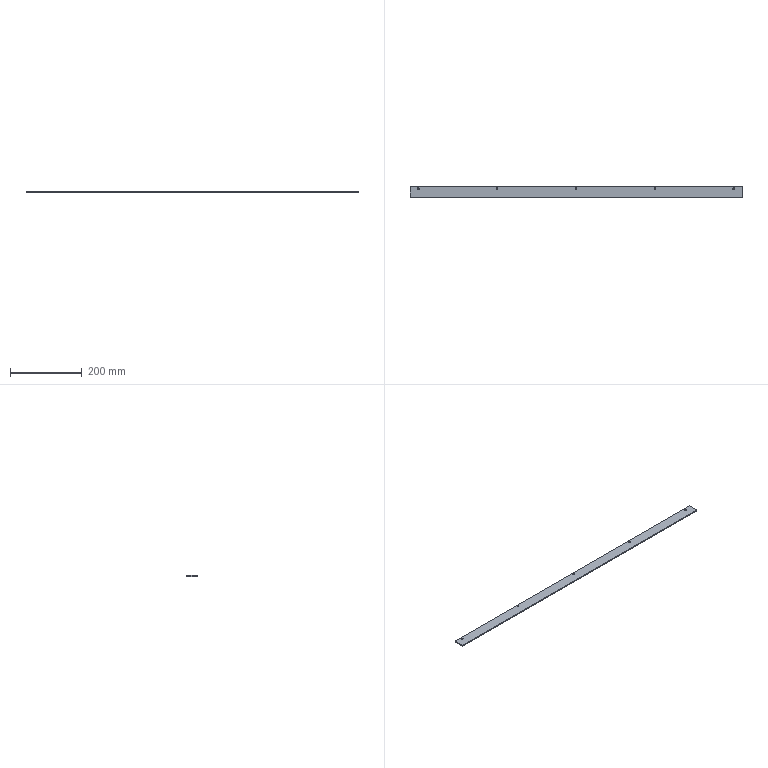Part | NX | features BREP 1 | 1 solid | 30 faces | box 926 x 30 x 3 mm | volume 82827 mm3 | plane 10 | cone 10 | cylinder 10 | commonest cylinder face diameters 4.8 x10
STEP:
#1=CARTESIAN_POINT('',(-463.,-14.,3.));
#2=VERTEX_POINT('',#1);
#3=CARTESIAN_POINT('',(-462.,-15.,3.));
#4=VERTEX_POINT('',#3);
#5=CARTESIAN_POINT('',(-238.5,-238.5,3.));
#6=DIRECTION('',(0.7071,-0.7071,0.));
#7=VECTOR('',#6,1000.);
#8=LINE('',#5,#7);
#9=EDGE_CURVE('',#2,#4,#8,.T.);
#10=ORIENTED_EDGE('',*,*,#9,.F.);
#11=CARTESIAN_POINT('',(-463.,-14.,0.));
#12=VERTEX_POINT('',#11);
#13=CARTESIAN_POINT('',(-463.,-14.,3.));
#14=DIRECTION('',(0.,0.,1.));
#15=VECTOR('',#14,1000.);
#16=LINE('',#13,#15);
#17=EDGE_CURVE('',#12,#2,#16,.T.);
#18=ORIENTED_EDGE('',*,*,#17,.F.);
#19=CARTESIAN_POINT('',(-462.,-15.,0.));
#20=VERTEX_POINT('',#19);
#21=CARTESIAN_POINT('',(-462.,-15.,0.));
#22=DIRECTION('',(-0.7071,0.7071,0.));
#23=VECTOR('',#22,1000.);
#24=LINE('',#21,#23);
#25=EDGE_CURVE('',#20,#12,#24,.T.);
#26=ORIENTED_EDGE('',*,*,#25,.F.);
#27=CARTESIAN_POINT('',(-462.,-15.,3.));
#28=DIRECTION('',(0.,0.,-1.));
#29=VECTOR('',#28,1000.);
#30=LINE('',#27,#29);
#31=EDGE_CURVE('',#4,#20,#30,.T.);
#32=ORIENTED_EDGE('',*,*,#31,.F.);
#33=EDGE_LOOP('',(#10,#18,#26,#32));
#34=FACE_BOUND('',#33,.T.);
#35=CARTESIAN_POINT('',(-462.,-15.,3.));
#36=DIRECTION('',(0.7071,0.7071,0.));
#37=DIRECTION('',(0.,0.,-1.));
#38=AXIS2_PLACEMENT_3D('',#35,#36,#37);
#39=PLANE('',#38);
#40=ADVANCED_FACE('',(#34),#39,.F.);
#41=CARTESIAN_POINT('',(-462.,15.,3.));
#42=VERTEX_POINT('',#41);
#43=CARTESIAN_POINT('',(-463.,14.,3.));
#44=VERTEX_POINT('',#43);
#45=CARTESIAN_POINT('',(-238.5,238.5,3.));
#46=DIRECTION('',(-0.7071,-0.7071,0.));
#47=VECTOR('',#46,1000.);
#48=LINE('',#45,#47);
#49=EDGE_CURVE('',#42,#44,#48,.T.);
#50=ORIENTED_EDGE('',*,*,#49,.F.);
#51=CARTESIAN_POINT('',(-462.,15.,0.));
#52=VERTEX_POINT('',#51);
#53=CARTESIAN_POINT('',(-462.,15.,3.));
#54=DIRECTION('',(0.,0.,1.));
#55=VECTOR('',#54,1000.);
#56=LINE('',#53,#55);
#57=EDGE_CURVE('',#52,#42,#56,.T.);
#58=ORIENTED_EDGE('',*,*,#57,.F.);
#59=CARTESIAN_POINT('',(-463.,14.,0.));
#60=VERTEX_POINT('',#59);
#61=CARTESIAN_POINT('',(-463.,14.,0.));
#62=DIRECTION('',(0.7071,0.7071,0.));
#63=VECTOR('',#62,1000.);
#64=LINE('',#61,#63);
#65=EDGE_CURVE('',#60,#52,#64,.T.);
#66=ORIENTED_EDGE('',*,*,#65,.F.);
#67=CARTESIAN_POINT('',(-463.,14.,3.));
#68=DIRECTION('',(0.,0.,-1.));
#69=VECTOR('',#68,1000.);
#70=LINE('',#67,#69);
#71=EDGE_CURVE('',#44,#60,#70,.T.);
#72=ORIENTED_EDGE('',*,*,#71,.F.);
#73=EDGE_LOOP('',(#50,#58,#66,#72));
#74=FACE_BOUND('',#73,.T.);
#75=CARTESIAN_POINT('',(-463.,14.,3.));
#76=DIRECTION('',(0.7071,-0.7071,0.));
#77=DIRECTION('',(0.,0.,-1.));
#78=AXIS2_PLACEMENT_3D('',#75,#76,#77);
#79=PLANE('',#78);
#80=ADVANCED_FACE('',(#74),#79,.F.);
#81=CARTESIAN_POINT('',(462.,-15.,3.));
#82=VERTEX_POINT('',#81);
#83=CARTESIAN_POINT('',(463.,-14.,3.));
#84=VERTEX_POINT('',#83);
#85=CARTESIAN_POINT('',(238.5,-238.5,3.));
#86=DIRECTION('',(0.7071,0.7071,0.));
#87=VECTOR('',#86,1000.);
#88=LINE('',#85,#87);
#89=EDGE_CURVE('',#82,#84,#88,.T.);
#90=ORIENTED_EDGE('',*,*,#89,.F.);
#91=CARTESIAN_POINT('',(462.,-15.,0.));
#92=VERTEX_POINT('',#91);
#93=CARTESIAN_POINT('',(462.,-15.,3.));
#94=DIRECTION('',(0.,0.,1.));
#95=VECTOR('',#94,1000.);
#96=LINE('',#93,#95);
#97=EDGE_CURVE('',#92,#82,#96,.T.);
#98=ORIENTED_EDGE('',*,*,#97,.F.);
#99=CARTESIAN_POINT('',(463.,-14.,0.));
#100=VERTEX_POINT('',#99);
#101=CARTESIAN_POINT('',(463.,-14.,0.));
#102=DIRECTION('',(-0.7071,-0.7071,0.));
#103=VECTOR('',#102,1000.);
#104=LINE('',#101,#103);
#105=EDGE_CURVE('',#100,#92,#104,.T.);
#106=ORIENTED_EDGE('',*,*,#105,.F.);
#107=CARTESIAN_POINT('',(463.,-14.,3.));
#108=DIRECTION('',(0.,0.,-1.));
#109=VECTOR('',#108,1000.);
#110=LINE('',#107,#109);
#111=EDGE_CURVE('',#84,#100,#110,.T.);
#112=ORIENTED_EDGE('',*,*,#111,.F.);
#113=EDGE_LOOP('',(#90,#98,#106,#112));
#114=FACE_BOUND('',#113,.T.);
#115=CARTESIAN_POINT('',(463.,-14.,3.));
#116=DIRECTION('',(-0.7071,0.7071,0.));
#117=DIRECTION('',(0.,0.,-1.));
#118=AXIS2_PLACEMENT_3D('',#115,#116,#117);
#119=PLANE('',#118);
#120=ADVANCED_FACE('',(#114),#119,.F.);
#121=CARTESIAN_POINT('',(463.,14.,3.));
#122=VERTEX_POINT('',#121);
#123=CARTESIAN_POINT('',(462.,15.,3.));
#124=VERTEX_POINT('',#123);
#125=CARTESIAN_POINT('',(238.5,238.5,3.));
#126=DIRECTION('',(-0.7071,0.7071,0.));
#127=VECTOR('',#126,1000.);
#128=LINE('',#125,#127);
#129=EDGE_CURVE('',#122,#124,#128,.T.);
#130=ORIENTED_EDGE('',*,*,#129,.F.);
#131=CARTESIAN_POINT('',(463.,14.,0.));
#132=VERTEX_POINT('',#131);
#133=CARTESIAN_POINT('',(463.,14.,3.));
#134=DIRECTION('',(0.,0.,1.));
#135=VECTOR('',#134,1000.);
#136=LINE('',#133,#135);
#137=EDGE_CURVE('',#132,#122,#136,.T.);
#138=ORIENTED_EDGE('',*,*,#137,.F.);
#139=CARTESIAN_POINT('',(462.,15.,0.));
#140=VERTEX_POINT('',#139);
#141=CARTESIAN_POINT('',(462.,15.,0.));
#142=DIRECTION('',(0.7071,-0.7071,0.));
#143=VECTOR('',#142,1000.);
#144=LINE('',#141,#143);
#145=EDGE_CURVE('',#140,#132,#144,.T.);
#146=ORIENTED_EDGE('',*,*,#145,.F.);
#147=CARTESIAN_POINT('',(462.,15.,3.));
#148=DIRECTION('',(0.,0.,-1.));
#149=VECTOR('',#148,1000.);
#150=LINE('',#147,#149);
#151=EDGE_CURVE('',#124,#140,#150,.T.);
#152=ORIENTED_EDGE('',*,*,#151,.F.);
#153=EDGE_LOOP('',(#130,#138,#146,#152));
#154=FACE_BOUND('',#153,.T.);
#155=CARTESIAN_POINT('',(462.,15.,3.));
#156=DIRECTION('',(-0.7071,-0.7071,0.));
#157=DIRECTION('',(0.,0.,-1.));
#158=AXIS2_PLACEMENT_3D('',#155,#156,#157);
#159=PLANE('',#158);
#160=ADVANCED_FACE('',(#154),#159,.F.);
#161=CARTESIAN_POINT('',(442.4,9.,2.19));
#162=VERTEX_POINT('',#161);
#163=CARTESIAN_POINT('',(444.59,9.,0.));
#164=VERTEX_POINT('',#163);
#165=CARTESIAN_POINT('',(444.59,9.,0.));
#166=DIRECTION('',(0.7071,0.,-0.7071));
#167=VECTOR('',#166,1000.);
#168=LINE('',#165,#167);
#169=EDGE_CURVE('',#162,#164,#168,.T.);
#170=ORIENTED_EDGE('',*,*,#169,.F.);
#171=CARTESIAN_POINT('',(437.6,9.,2.19));
#172=VERTEX_POINT('',#171);
#173=CARTESIAN_POINT('',(440.,9.,2.19));
#174=DIRECTION('',(0.,0.,-1.));
#175=DIRECTION('',(-1.,0.,0.));
#176=AXIS2_PLACEMENT_3D('',#173,#174,#175);
#177=CIRCLE('',#176,2.4);
#178=EDGE_CURVE('',#172,#162,#177,.T.);
#179=ORIENTED_EDGE('',*,*,#178,.F.);
#180=CARTESIAN_POINT('',(435.41,9.,0.));
#181=VERTEX_POINT('',#180);
#182=CARTESIAN_POINT('',(435.41,9.,0.));
#183=DIRECTION('',(-0.7071,0.,-0.7071));
#184=VECTOR('',#183,1000.);
#185=LINE('',#182,#184);
#186=EDGE_CURVE('',#172,#181,#185,.T.);
#187=ORIENTED_EDGE('',*,*,#186,.T.);
#188=CARTESIAN_POINT('',(440.,9.,0.));
#189=DIRECTION('',(0.,0.,-1.));
#190=DIRECTION('',(-1.,0.,0.));
#191=AXIS2_PLACEMENT_3D('',#188,#189,#190);
#192=CIRCLE('',#191,4.59);
#193=EDGE_CURVE('',#181,#164,#192,.T.);
#194=ORIENTED_EDGE('',*,*,#193,.T.);
#195=EDGE_LOOP('',(#170,#179,#187,#194));
#196=FACE_BOUND('',#195,.T.);
#197=CARTESIAN_POINT('',(440.,9.,0.));
#198=DIRECTION('',(0.,0.,-1.));
#199=DIRECTION('',(-1.,0.,0.));
#200=AXIS2_PLACEMENT_3D('',#197,#198,#199);
#201=CONICAL_SURFACE('',#200,4.59,0.7854);
#202=ADVANCED_FACE('',(#196),#201,.F.);
#203=CARTESIAN_POINT('',(442.4,9.,3.));
#204=VERTEX_POINT('',#203);
#205=CARTESIAN_POINT('',(442.4,9.,0.));
#206=DIRECTION('',(0.,0.,-1.));
#207=VECTOR('',#206,1000.);
#208=LINE('',#205,#207);
#209=EDGE_CURVE('',#204,#162,#208,.T.);
#210=ORIENTED_EDGE('',*,*,#209,.F.);
#211=CARTESIAN_POINT('',(437.6,9.,3.));
#212=VERTEX_POINT('',#211);
#213=CARTESIAN_POINT('',(440.,9.,3.));
#214=DIRECTION('',(0.,0.,-1.));
#215=DIRECTION('',(-1.,0.,0.));
#216=AXIS2_PLACEMENT_3D('',#213,#214,#215);
#217=CIRCLE('',#216,2.4);
#218=EDGE_CURVE('',#212,#204,#217,.T.);
#219=ORIENTED_EDGE('',*,*,#218,.F.);
#220=CARTESIAN_POINT('',(437.6,9.,0.));
#221=DIRECTION('',(0.,0.,-1.));
#222=VECTOR('',#221,1000.);
#223=LINE('',#220,#222);
#224=EDGE_CURVE('',#212,#172,#223,.T.);
#225=ORIENTED_EDGE('',*,*,#224,.T.);
#226=ORIENTED_EDGE('',*,*,#178,.T.);
#227=EDGE_LOOP('',(#210,#219,#225,#226));
#228=FACE_BOUND('',#227,.T.);
#229=CARTESIAN_POINT('',(440.,9.,0.));
#230=DIRECTION('',(0.,0.,-1.));
#231=DIRECTION('',(-1.,0.,0.));
#232=AXIS2_PLACEMENT_3D('',#229,#230,#231);
#233=CYLINDRICAL_SURFACE('',#232,2.4);
#234=ADVANCED_FACE('',(#228),#233,.F.);
#235=CARTESIAN_POINT('',(222.4,9.,2.19));
#236=VERTEX_POINT('',#235);
#237=CARTESIAN_POINT('',(224.59,9.,0.));
#238=VERTEX_POINT('',#237);
#239=CARTESIAN_POINT('',(224.59,9.,0.));
#240=DIRECTION('',(0.7071,0.,-0.7071));
#241=VECTOR('',#240,1000.);
#242=LINE('',#239,#241);
#243=EDGE_CURVE('',#236,#238,#242,.T.);
#244=ORIENTED_EDGE('',*,*,#243,.F.);
#245=CARTESIAN_POINT('',(217.6,9.,2.19));
#246=VERTEX_POINT('',#245);
#247=CARTESIAN_POINT('',(220.,9.,2.19));
#248=DIRECTION('',(0.,0.,-1.));
#249=DIRECTION('',(-1.,0.,0.));
#250=AXIS2_PLACEMENT_3D('',#247,#248,#249);
#251=CIRCLE('',#250,2.4);
#252=EDGE_CURVE('',#246,#236,#251,.T.);
#253=ORIENTED_EDGE('',*,*,#252,.F.);
#254=CARTESIAN_POINT('',(215.41,9.,0.));
#255=VERTEX_POINT('',#254);
#256=CARTESIAN_POINT('',(215.41,9.,0.));
#257=DIRECTION('',(-0.7071,0.,-0.7071));
#258=VECTOR('',#257,1000.);
#259=LINE('',#256,#258);
#260=EDGE_CURVE('',#246,#255,#259,.T.);
#261=ORIENTED_EDGE('',*,*,#260,.T.);
#262=CARTESIAN_POINT('',(220.,9.,0.));
#263=DIRECTION('',(0.,0.,-1.));
#264=DIRECTION('',(-1.,0.,0.));
#265=AXIS2_PLACEMENT_3D('',#262,#263,#264);
#266=CIRCLE('',#265,4.59);
#267=EDGE_CURVE('',#255,#238,#266,.T.);
#268=ORIENTED_EDGE('',*,*,#267,.T.);
#269=EDGE_LOOP('',(#244,#253,#261,#268));
#270=FACE_BOUND('',#269,.T.);
#271=CARTESIAN_POINT('',(220.,9.,0.));
#272=DIRECTION('',(0.,0.,-1.));
#273=DIRECTION('',(-1.,0.,0.));
#274=AXIS2_PLACEMENT_3D('',#271,#272,#273);
#275=CONICAL_SURFACE('',#274,4.59,0.7854);
#276=ADVANCED_FACE('',(#270),#275,.F.);
#277=CARTESIAN_POINT('',(222.4,9.,3.));
#278=VERTEX_POINT('',#277);
#279=CARTESIAN_POINT('',(222.4,9.,0.));
#280=DIRECTION('',(0.,0.,-1.));
#281=VECTOR('',#280,1000.);
#282=LINE('',#279,#281);
#283=EDGE_CURVE('',#278,#236,#282,.T.);
#284=ORIENTED_EDGE('',*,*,#283,.F.);
#285=CARTESIAN_POINT('',(217.6,9.,3.));
#286=VERTEX_POINT('',#285);
#287=CARTESIAN_POINT('',(220.,9.,3.));
#288=DIRECTION('',(0.,0.,-1.));
#289=DIRECTION('',(-1.,0.,0.));
#290=AXIS2_PLACEMENT_3D('',#287,#288,#289);
#291=CIRCLE('',#290,2.4);
#292=EDGE_CURVE('',#286,#278,#291,.T.);
#293=ORIENTED_EDGE('',*,*,#292,.F.);
#294=CARTESIAN_POINT('',(217.6,9.,0.));
#295=DIRECTION('',(0.,0.,-1.));
#296=VECTOR('',#295,1000.);
#297=LINE('',#294,#296);
#298=EDGE_CURVE('',#286,#246,#297,.T.);
#299=ORIENTED_EDGE('',*,*,#298,.T.);
#300=ORIENTED_EDGE('',*,*,#252,.T.);
#301=EDGE_LOOP('',(#284,#293,#299,#300));
#302=FACE_BOUND('',#301,.T.);
#303=CARTESIAN_POINT('',(220.,9.,0.));
#304=DIRECTION('',(0.,0.,-1.));
#305=DIRECTION('',(-1.,0.,0.));
#306=AXIS2_PLACEMENT_3D('',#303,#304,#305);
#307=CYLINDRICAL_SURFACE('',#306,2.4);
#308=ADVANCED_FACE('',(#302),#307,.F.);
#309=CARTESIAN_POINT('',(2.4,9.,2.19));
#310=VERTEX_POINT('',#309);
#311=CARTESIAN_POINT('',(4.59,9.,0.));
#312=VERTEX_POINT('',#311);
#313=CARTESIAN_POINT('',(4.59,9.,0.));
#314=DIRECTION('',(0.7071,0.,-0.7071));
#315=VECTOR('',#314,1000.);
#316=LINE('',#313,#315);
#317=EDGE_CURVE('',#310,#312,#316,.T.);
#318=ORIENTED_EDGE('',*,*,#317,.F.);
#319=CARTESIAN_POINT('',(-2.4,9.,2.19));
#320=VERTEX_POINT('',#319);
#321=CARTESIAN_POINT('',(0.,9.,2.19));
#322=DIRECTION('',(0.,0.,-1.));
#323=DIRECTION('',(-1.,0.,0.));
#324=AXIS2_PLACEMENT_3D('',#321,#322,#323);
#325=CIRCLE('',#324,2.4);
#326=EDGE_CURVE('',#320,#310,#325,.T.);
#327=ORIENTED_EDGE('',*,*,#326,.F.);
#328=CARTESIAN_POINT('',(-4.59,9.,0.));
#329=VERTEX_POINT('',#328);
#330=CARTESIAN_POINT('',(-4.59,9.,0.));
#331=DIRECTION('',(-0.7071,0.,-0.7071));
#332=VECTOR('',#331,1000.);
#333=LINE('',#330,#332);
#334=EDGE_CURVE('',#320,#329,#333,.T.);
#335=ORIENTED_EDGE('',*,*,#334,.T.);
#336=CARTESIAN_POINT('',(0.,9.,0.));
#337=DIRECTION('',(0.,0.,-1.));
#338=DIRECTION('',(-1.,0.,0.));
#339=AXIS2_PLACEMENT_3D('',#336,#337,#338);
#340=CIRCLE('',#339,4.59);
#341=EDGE_CURVE('',#329,#312,#340,.T.);
#342=ORIENTED_EDGE('',*,*,#341,.T.);
#343=EDGE_LOOP('',(#318,#327,#335,#342));
#344=FACE_BOUND('',#343,.T.);
#345=CARTESIAN_POINT('',(0.,9.,0.));
#346=DIRECTION('',(0.,0.,-1.));
#347=DIRECTION('',(-1.,0.,0.));
#348=AXIS2_PLACEMENT_3D('',#345,#346,#347);
#349=CONICAL_SURFACE('',#348,4.59,0.7854);
#350=ADVANCED_FACE('',(#344),#349,.F.);
#351=CARTESIAN_POINT('',(2.4,9.,3.));
#352=VERTEX_POINT('',#351);
#353=CARTESIAN_POINT('',(2.4,9.,0.));
#354=DIRECTION('',(0.,0.,-1.));
#355=VECTOR('',#354,1000.);
#356=LINE('',#353,#355);
#357=EDGE_CURVE('',#352,#310,#356,.T.);
#358=ORIENTED_EDGE('',*,*,#357,.F.);
#359=CARTESIAN_POINT('',(-2.4,9.,3.));
#360=VERTEX_POINT('',#359);
#361=CARTESIAN_POINT('',(0.,9.,3.));
#362=DIRECTION('',(0.,0.,-1.));
#363=DIRECTION('',(-1.,0.,0.));
#364=AXIS2_PLACEMENT_3D('',#361,#362,#363);
#365=CIRCLE('',#364,2.4);
#366=EDGE_CURVE('',#360,#352,#365,.T.);
#367=ORIENTED_EDGE('',*,*,#366,.F.);
#368=CARTESIAN_POINT('',(-2.4,9.,0.));
#369=DIRECTION('',(0.,0.,-1.));
#370=VECTOR('',#369,1000.);
#371=LINE('',#368,#370);
#372=EDGE_CURVE('',#360,#320,#371,.T.);
#373=ORIENTED_EDGE('',*,*,#372,.T.);
#374=ORIENTED_EDGE('',*,*,#326,.T.);
#375=EDGE_LOOP('',(#358,#367,#373,#374));
#376=FACE_BOUND('',#375,.T.);
#377=CARTESIAN_POINT('',(0.,9.,0.));
#378=DIRECTION('',(0.,0.,-1.));
#379=DIRECTION('',(-1.,0.,0.));
#380=AXIS2_PLACEMENT_3D('',#377,#378,#379);
#381=CYLINDRICAL_SURFACE('',#380,2.4);
#382=ADVANCED_FACE('',(#376),#381,.F.);
#383=CARTESIAN_POINT('',(-217.6,9.,2.19));
#384=VERTEX_POINT('',#383);
#385=CARTESIAN_POINT('',(-215.41,9.,0.));
#386=VERTEX_POINT('',#385);
#387=CARTESIAN_POINT('',(-215.41,9.,0.));
#388=DIRECTION('',(0.7071,0.,-0.7071));
#389=VECTOR('',#388,1000.);
#390=LINE('',#387,#389);
#391=EDGE_CURVE('',#384,#386,#390,.T.);
#392=ORIENTED_EDGE('',*,*,#391,.F.);
#393=CARTESIAN_POINT('',(-222.4,9.,2.19));
#394=VERTEX_POINT('',#393);
#395=CARTESIAN_POINT('',(-220.,9.,2.19));
#396=DIRECTION('',(0.,0.,-1.));
#397=DIRECTION('',(-1.,0.,0.));
#398=AXIS2_PLACEMENT_3D('',#395,#396,#397);
#399=CIRCLE('',#398,2.4);
#400=EDGE_CURVE('',#394,#384,#399,.T.);
#401=ORIENTED_EDGE('',*,*,#400,.F.);
#402=CARTESIAN_POINT('',(-224.59,9.,0.));
#403=VERTEX_POINT('',#402);
#404=CARTESIAN_POINT('',(-224.59,9.,0.));
#405=DIRECTION('',(-0.7071,0.,-0.7071));
#406=VECTOR('',#405,1000.);
#407=LINE('',#404,#406);
#408=EDGE_CURVE('',#394,#403,#407,.T.);
#409=ORIENTED_EDGE('',*,*,#408,.T.);
#410=CARTESIAN_POINT('',(-220.,9.,0.));
#411=DIRECTION('',(0.,0.,-1.));
#412=DIRECTION('',(-1.,0.,0.));
#413=AXIS2_PLACEMENT_3D('',#410,#411,#412);
#414=CIRCLE('',#413,4.59);
#415=EDGE_CURVE('',#403,#386,#414,.T.);
#416=ORIENTED_EDGE('',*,*,#415,.T.);
#417=EDGE_LOOP('',(#392,#401,#409,#416));
#418=FACE_BOUND('',#417,.T.);
#419=CARTESIAN_POINT('',(-220.,9.,0.));
#420=DIRECTION('',(0.,0.,-1.));
#421=DIRECTION('',(-1.,0.,0.));
#422=AXIS2_PLACEMENT_3D('',#419,#420,#421);
#423=CONICAL_SURFACE('',#422,4.59,0.7854);
#424=ADVANCED_FACE('',(#418),#423,.F.);
#425=CARTESIAN_POINT('',(-217.6,9.,3.));
#426=VERTEX_POINT('',#425);
#427=CARTESIAN_POINT('',(-217.6,9.,0.));
#428=DIRECTION('',(0.,0.,-1.));
#429=VECTOR('',#428,1000.);
#430=LINE('',#427,#429);
#431=EDGE_CURVE('',#426,#384,#430,.T.);
#432=ORIENTED_EDGE('',*,*,#431,.F.);
#433=CARTESIAN_POINT('',(-222.4,9.,3.));
#434=VERTEX_POINT('',#433);
#435=CARTESIAN_POINT('',(-220.,9.,3.));
#436=DIRECTION('',(0.,0.,-1.));
#437=DIRECTION('',(-1.,0.,0.));
#438=AXIS2_PLACEMENT_3D('',#435,#436,#437);
#439=CIRCLE('',#438,2.4);
#440=EDGE_CURVE('',#434,#426,#439,.T.);
#441=ORIENTED_EDGE('',*,*,#440,.F.);
#442=CARTESIAN_POINT('',(-222.4,9.,0.));
#443=DIRECTION('',(0.,0.,-1.));
#444=VECTOR('',#443,1000.);
#445=LINE('',#442,#444);
#446=EDGE_CURVE('',#434,#394,#445,.T.);
#447=ORIENTED_EDGE('',*,*,#446,.T.);
#448=ORIENTED_EDGE('',*,*,#400,.T.);
#449=EDGE_LOOP('',(#432,#441,#447,#448));
#450=FACE_BOUND('',#449,.T.);
#451=CARTESIAN_POINT('',(-220.,9.,0.));
#452=DIRECTION('',(0.,0.,-1.));
#453=DIRECTION('',(-1.,0.,0.));
#454=AXIS2_PLACEMENT_3D('',#451,#452,#453);
#455=CYLINDRICAL_SURFACE('',#454,2.4);
#456=ADVANCED_FACE('',(#450),#455,.F.);
#457=CARTESIAN_POINT('',(-437.6,9.,2.19));
#458=VERTEX_POINT('',#457);
#459=CARTESIAN_POINT('',(-435.41,9.,0.));
#460=VERTEX_POINT('',#459);
#461=CARTESIAN_POINT('',(-435.41,9.,0.));
#462=DIRECTION('',(0.7071,0.,-0.7071));
#463=VECTOR('',#462,1000.);
#464=LINE('',#461,#463);
#465=EDGE_CURVE('',#458,#460,#464,.T.);
#466=ORIENTED_EDGE('',*,*,#465,.F.);
#467=CARTESIAN_POINT('',(-442.4,9.,2.19));
#468=VERTEX_POINT('',#467);
#469=CARTESIAN_POINT('',(-440.,9.,2.19));
#470=DIRECTION('',(0.,0.,-1.));
#471=DIRECTION('',(-1.,0.,0.));
#472=AXIS2_PLACEMENT_3D('',#469,#470,#471);
#473=CIRCLE('',#472,2.4);
#474=EDGE_CURVE('',#468,#458,#473,.T.);
#475=ORIENTED_EDGE('',*,*,#474,.F.);
#476=CARTESIAN_POINT('',(-444.59,9.,0.));
#477=VERTEX_POINT('',#476);
#478=CARTESIAN_POINT('',(-444.59,9.,0.));
#479=DIRECTION('',(-0.7071,0.,-0.7071));
#480=VECTOR('',#479,1000.);
#481=LINE('',#478,#480);
#482=EDGE_CURVE('',#468,#477,#481,.T.);
#483=ORIENTED_EDGE('',*,*,#482,.T.);
#484=CARTESIAN_POINT('',(-440.,9.,0.));
#485=DIRECTION('',(0.,0.,-1.));
#486=DIRECTION('',(-1.,0.,0.));
#487=AXIS2_PLACEMENT_3D('',#484,#485,#486);
#488=CIRCLE('',#487,4.59);
#489=EDGE_CURVE('',#477,#460,#488,.T.);
#490=ORIENTED_EDGE('',*,*,#489,.T.);
#491=EDGE_LOOP('',(#466,#475,#483,#490));
#492=FACE_BOUND('',#491,.T.);
#493=CARTESIAN_POINT('',(-440.,9.,0.));
#494=DIRECTION('',(0.,0.,-1.));
#495=DIRECTION('',(-1.,0.,0.));
#496=AXIS2_PLACEMENT_3D('',#493,#494,#495);
#497=CONICAL_SURFACE('',#496,4.59,0.7854);
#498=ADVANCED_FACE('',(#492),#497,.F.);
#499=CARTESIAN_POINT('',(-437.6,9.,3.));
#500=VERTEX_POINT('',#499);
#501=CARTESIAN_POINT('',(-437.6,9.,0.));
#502=DIRECTION('',(0.,0.,-1.));
#503=VECTOR('',#502,1000.);
#504=LINE('',#501,#503);
#505=EDGE_CURVE('',#500,#458,#504,.T.);
#506=ORIENTED_EDGE('',*,*,#505,.F.);
#507=CARTESIAN_POINT('',(-442.4,9.,3.));
#508=VERTEX_POINT('',#507);
#509=CARTESIAN_POINT('',(-440.,9.,3.));
#510=DIRECTION('',(0.,0.,-1.));
#511=DIRECTION('',(-1.,0.,0.));
#512=AXIS2_PLACEMENT_3D('',#509,#510,#511);
#513=CIRCLE('',#512,2.4);
#514=EDGE_CURVE('',#508,#500,#513,.T.);
#515=ORIENTED_EDGE('',*,*,#514,.F.);
#516=CARTESIAN_POINT('',(-442.4,9.,0.));
#517=DIRECTION('',(0.,0.,-1.));
#518=VECTOR('',#517,1000.);
#519=LINE('',#516,#518);
#520=EDGE_CURVE('',#508,#468,#519,.T.);
#521=ORIENTED_EDGE('',*,*,#520,.T.);
#522=ORIENTED_EDGE('',*,*,#474,.T.);
#523=EDGE_LOOP('',(#506,#515,#521,#522));
#524=FACE_BOUND('',#523,.T.);
#525=CARTESIAN_POINT('',(-440.,9.,0.));
#526=DIRECTION('',(0.,0.,-1.));
#527=DIRECTION('',(-1.,0.,0.));
#528=AXIS2_PLACEMENT_3D('',#525,#526,#527);
#529=CYLINDRICAL_SURFACE('',#528,2.4);
#530=ADVANCED_FACE('',(#524),#529,.F.);
#531=CARTESIAN_POINT('',(463.,15.,0.));
#532=DIRECTION('',(-1.,0.,0.));
#533=VECTOR('',#532,1000.);
#534=LINE('',#531,#533);
#535=EDGE_CURVE('',#140,#52,#534,.T.);
#536=ORIENTED_EDGE('',*,*,#535,.F.);
#537=ORIENTED_EDGE('',*,*,#145,.T.);
#538=CARTESIAN_POINT('',(463.,-15.,0.));
#539=DIRECTION('',(0.,1.,0.));
#540=VECTOR('',#539,1000.);
#541=LINE('',#538,#540);
#542=EDGE_CURVE('',#100,#132,#541,.T.);
#543=ORIENTED_EDGE('',*,*,#542,.F.);
#544=ORIENTED_EDGE('',*,*,#105,.T.);
#545=CARTESIAN_POINT('',(463.,-15.,0.));
#546=DIRECTION('',(1.,0.,0.));
#547=VECTOR('',#546,1000.);
#548=LINE('',#545,#547);
#549=EDGE_CURVE('',#20,#92,#548,.T.);
#550=ORIENTED_EDGE('',*,*,#549,.F.);
#551=ORIENTED_EDGE('',*,*,#25,.T.);
#552=CARTESIAN_POINT('',(-463.,-15.,0.));
#553=DIRECTION('',(0.,-1.,0.));
#554=VECTOR('',#553,1000.);
#555=LINE('',#552,#554);
#556=EDGE_CURVE('',#60,#12,#555,.T.);
#557=ORIENTED_EDGE('',*,*,#556,.F.);
#558=ORIENTED_EDGE('',*,*,#65,.T.);
#559=EDGE_LOOP('',(#536,#537,#543,#544,#550,#551,#557,#558));
#560=FACE_BOUND('',#559,.T.);
#561=ORIENTED_EDGE('',*,*,#489,.F.);
#562=CARTESIAN_POINT('',(-440.,9.,0.));
#563=DIRECTION('',(0.,0.,-1.));
#564=DIRECTION('',(-1.,0.,0.));
#565=AXIS2_PLACEMENT_3D('',#562,#563,#564);
#566=CIRCLE('',#565,4.59);
#567=EDGE_CURVE('',#460,#477,#566,.T.);
#568=ORIENTED_EDGE('',*,*,#567,.F.);
#569=EDGE_LOOP('',(#561,#568));
#570=FACE_BOUND('',#569,.T.);
#571=ORIENTED_EDGE('',*,*,#415,.F.);
#572=CARTESIAN_POINT('',(-220.,9.,0.));
#573=DIRECTION('',(0.,0.,-1.));
#574=DIRECTION('',(-1.,0.,0.));
#575=AXIS2_PLACEMENT_3D('',#572,#573,#574);
#576=CIRCLE('',#575,4.59);
#577=EDGE_CURVE('',#386,#403,#576,.T.);
#578=ORIENTED_EDGE('',*,*,#577,.F.);
#579=EDGE_LOOP('',(#571,#578));
#580=FACE_BOUND('',#579,.T.);
#581=ORIENTED_EDGE('',*,*,#341,.F.);
#582=CARTESIAN_POINT('',(0.,9.,0.));
#583=DIRECTION('',(0.,0.,-1.));
#584=DIRECTION('',(-1.,0.,0.));
#585=AXIS2_PLACEMENT_3D('',#582,#583,#584);
#586=CIRCLE('',#585,4.59);
#587=EDGE_CURVE('',#312,#329,#586,.T.);
#588=ORIENTED_EDGE('',*,*,#587,.F.);
#589=EDGE_LOOP('',(#581,#588));
#590=FACE_BOUND('',#589,.T.);
#591=ORIENTED_EDGE('',*,*,#267,.F.);
#592=CARTESIAN_POINT('',(220.,9.,0.));
#593=DIRECTION('',(0.,0.,-1.));
#594=DIRECTION('',(-1.,0.,0.));
#595=AXIS2_PLACEMENT_3D('',#592,#593,#594);
#596=CIRCLE('',#595,4.59);
#597=EDGE_CURVE('',#238,#255,#596,.T.);
#598=ORIENTED_EDGE('',*,*,#597,.F.);
#599=EDGE_LOOP('',(#591,#598));
#600=FACE_BOUND('',#599,.T.);
#601=ORIENTED_EDGE('',*,*,#193,.F.);
#602=CARTESIAN_POINT('',(440.,9.,0.));
#603=DIRECTION('',(0.,0.,-1.));
#604=DIRECTION('',(-1.,0.,0.));
#605=AXIS2_PLACEMENT_3D('',#602,#603,#604);
#606=CIRCLE('',#605,4.59);
#607=EDGE_CURVE('',#164,#181,#606,.T.);
#608=ORIENTED_EDGE('',*,*,#607,.F.);
#609=EDGE_LOOP('',(#601,#608));
#610=FACE_BOUND('',#609,.T.);
#611=CARTESIAN_POINT('',(0.,0.,0.));
#612=DIRECTION('',(0.,0.,1.));
#613=DIRECTION('',(1.,0.,0.));
#614=AXIS2_PLACEMENT_3D('',#611,#612,#613);
#615=PLANE('',#614);
#616=ADVANCED_FACE('',(#560,#570,#580,#590,#600,#610),#615,.F.);
#617=CARTESIAN_POINT('',(463.,-15.,3.));
#618=DIRECTION('',(0.,1.,0.));
#619=VECTOR('',#618,1000.);
#620=LINE('',#617,#619);
#621=EDGE_CURVE('',#84,#122,#620,.T.);
#622=ORIENTED_EDGE('',*,*,#621,.T.);
#623=ORIENTED_EDGE('',*,*,#129,.T.);
#624=CARTESIAN_POINT('',(463.,15.,3.));
#625=DIRECTION('',(-1.,0.,0.));
#626=VECTOR('',#625,1000.);
#627=LINE('',#624,#626);
#628=EDGE_CURVE('',#124,#42,#627,.T.);
#629=ORIENTED_EDGE('',*,*,#628,.T.);
#630=ORIENTED_EDGE('',*,*,#49,.T.);
#631=CARTESIAN_POINT('',(-463.,-15.,3.));
#632=DIRECTION('',(0.,-1.,0.));
#633=VECTOR('',#632,1000.);
#634=LINE('',#631,#633);
#635=EDGE_CURVE('',#44,#2,#634,.T.);
#636=ORIENTED_EDGE('',*,*,#635,.T.);
#637=ORIENTED_EDGE('',*,*,#9,.T.);
#638=CARTESIAN_POINT('',(463.,-15.,3.));
#639=DIRECTION('',(1.,0.,0.));
#640=VECTOR('',#639,1000.);
#641=LINE('',#638,#640);
#642=EDGE_CURVE('',#4,#82,#641,.T.);
#643=ORIENTED_EDGE('',*,*,#642,.T.);
#644=ORIENTED_EDGE('',*,*,#89,.T.);
#645=EDGE_LOOP('',(#622,#623,#629,#630,#636,#637,#643,#644));
#646=FACE_BOUND('',#645,.T.);
#647=ORIENTED_EDGE('',*,*,#514,.T.);
#648=CARTESIAN_POINT('',(-440.,9.,3.));
#649=DIRECTION('',(0.,0.,-1.));
#650=DIRECTION('',(-1.,0.,0.));
#651=AXIS2_PLACEMENT_3D('',#648,#649,#650);
#652=CIRCLE('',#651,2.4);
#653=EDGE_CURVE('',#500,#508,#652,.T.);
#654=ORIENTED_EDGE('',*,*,#653,.T.);
#655=EDGE_LOOP('',(#647,#654));
#656=FACE_BOUND('',#655,.T.);
#657=ORIENTED_EDGE('',*,*,#440,.T.);
#658=CARTESIAN_POINT('',(-220.,9.,3.));
#659=DIRECTION('',(0.,0.,-1.));
#660=DIRECTION('',(-1.,0.,0.));
#661=AXIS2_PLACEMENT_3D('',#658,#659,#660);
#662=CIRCLE('',#661,2.4);
#663=EDGE_CURVE('',#426,#434,#662,.T.);
#664=ORIENTED_EDGE('',*,*,#663,.T.);
#665=EDGE_LOOP('',(#657,#664));
#666=FACE_BOUND('',#665,.T.);
#667=ORIENTED_EDGE('',*,*,#366,.T.);
#668=CARTESIAN_POINT('',(0.,9.,3.));
#669=DIRECTION('',(0.,0.,-1.));
#670=DIRECTION('',(-1.,0.,0.));
#671=AXIS2_PLACEMENT_3D('',#668,#669,#670);
#672=CIRCLE('',#671,2.4);
#673=EDGE_CURVE('',#352,#360,#672,.T.);
#674=ORIENTED_EDGE('',*,*,#673,.T.);
#675=EDGE_LOOP('',(#667,#674));
#676=FACE_BOUND('',#675,.T.);
#677=ORIENTED_EDGE('',*,*,#292,.T.);
#678=CARTESIAN_POINT('',(220.,9.,3.));
#679=DIRECTION('',(0.,0.,-1.));
#680=DIRECTION('',(-1.,0.,0.));
#681=AXIS2_PLACEMENT_3D('',#678,#679,#680);
#682=CIRCLE('',#681,2.4);
#683=EDGE_CURVE('',#278,#286,#682,.T.);
#684=ORIENTED_EDGE('',*,*,#683,.T.);
#685=EDGE_LOOP('',(#677,#684));
#686=FACE_BOUND('',#685,.T.);
#687=ORIENTED_EDGE('',*,*,#218,.T.);
#688=CARTESIAN_POINT('',(440.,9.,3.));
#689=DIRECTION('',(0.,0.,-1.));
#690=DIRECTION('',(-1.,0.,0.));
#691=AXIS2_PLACEMENT_3D('',#688,#689,#690);
#692=CIRCLE('',#691,2.4);
#693=EDGE_CURVE('',#204,#212,#692,.T.);
#694=ORIENTED_EDGE('',*,*,#693,.T.);
#695=EDGE_LOOP('',(#687,#694));
#696=FACE_BOUND('',#695,.T.);
#697=CARTESIAN_POINT('',(0.,0.,3.));
#698=DIRECTION('',(0.,0.,1.));
#699=DIRECTION('',(1.,0.,0.));
#700=AXIS2_PLACEMENT_3D('',#697,#698,#699);
#701=PLANE('',#700);
#702=ADVANCED_FACE('',(#646,#656,#666,#676,#686,#696),#701,.T.);
#703=ORIENTED_EDGE('',*,*,#628,.F.);
#704=ORIENTED_EDGE('',*,*,#151,.T.);
#705=ORIENTED_EDGE('',*,*,#535,.T.);
#706=ORIENTED_EDGE('',*,*,#57,.T.);
#707=EDGE_LOOP('',(#703,#704,#705,#706));
#708=FACE_BOUND('',#707,.T.);
#709=CARTESIAN_POINT('',(463.,15.,3.));
#710=DIRECTION('',(0.,-1.,0.));
#711=DIRECTION('',(1.,0.,0.));
#712=AXIS2_PLACEMENT_3D('',#709,#710,#711);
#713=PLANE('',#712);
#714=ADVANCED_FACE('',(#708),#713,.F.);
#715=ORIENTED_EDGE('',*,*,#542,.T.);
#716=ORIENTED_EDGE('',*,*,#137,.T.);
#717=ORIENTED_EDGE('',*,*,#621,.F.);
#718=ORIENTED_EDGE('',*,*,#111,.T.);
#719=EDGE_LOOP('',(#715,#716,#717,#718));
#720=FACE_BOUND('',#719,.T.);
#721=CARTESIAN_POINT('',(463.,-15.,3.));
#722=DIRECTION('',(-1.,0.,0.));
#723=DIRECTION('',(0.,0.,1.));
#724=AXIS2_PLACEMENT_3D('',#721,#722,#723);
#725=PLANE('',#724);
#726=ADVANCED_FACE('',(#720),#725,.F.);
#727=ORIENTED_EDGE('',*,*,#549,.T.);
#728=ORIENTED_EDGE('',*,*,#97,.T.);
#729=ORIENTED_EDGE('',*,*,#642,.F.);
#730=ORIENTED_EDGE('',*,*,#31,.T.);
#731=EDGE_LOOP('',(#727,#728,#729,#730));
#732=FACE_BOUND('',#731,.T.);
#733=CARTESIAN_POINT('',(463.,-15.,3.));
#734=DIRECTION('',(0.,1.,0.));
#735=DIRECTION('',(-1.,0.,0.));
#736=AXIS2_PLACEMENT_3D('',#733,#734,#735);
#737=PLANE('',#736);
#738=ADVANCED_FACE('',(#732),#737,.F.);
#739=ORIENTED_EDGE('',*,*,#635,.F.);
#740=ORIENTED_EDGE('',*,*,#71,.T.);
#741=ORIENTED_EDGE('',*,*,#556,.T.);
#742=ORIENTED_EDGE('',*,*,#17,.T.);
#743=EDGE_LOOP('',(#739,#740,#741,#742));
#744=FACE_BOUND('',#743,.T.);
#745=CARTESIAN_POINT('',(-463.,-15.,3.));
#746=DIRECTION('',(1.,0.,0.));
#747=DIRECTION('',(0.,0.,-1.));
#748=AXIS2_PLACEMENT_3D('',#745,#746,#747);
#749=PLANE('',#748);
#750=ADVANCED_FACE('',(#744),#749,.F.);
#751=ORIENTED_EDGE('',*,*,#653,.F.);
#752=ORIENTED_EDGE('',*,*,#505,.T.);
#753=CARTESIAN_POINT('',(-440.,9.,2.19));
#754=DIRECTION('',(0.,0.,-1.));
#755=DIRECTION('',(-1.,0.,0.));
#756=AXIS2_PLACEMENT_3D('',#753,#754,#755);
#757=CIRCLE('',#756,2.4);
#758=EDGE_CURVE('',#458,#468,#757,.T.);
#759=ORIENTED_EDGE('',*,*,#758,.T.);
#760=ORIENTED_EDGE('',*,*,#520,.F.);
#761=EDGE_LOOP('',(#751,#752,#759,#760));
#762=FACE_BOUND('',#761,.T.);
#763=CARTESIAN_POINT('',(-440.,9.,0.));
#764=DIRECTION('',(0.,0.,-1.));
#765=DIRECTION('',(-1.,0.,0.));
#766=AXIS2_PLACEMENT_3D('',#763,#764,#765);
#767=CYLINDRICAL_SURFACE('',#766,2.4);
#768=ADVANCED_FACE('',(#762),#767,.F.);
#769=ORIENTED_EDGE('',*,*,#758,.F.);
#770=ORIENTED_EDGE('',*,*,#465,.T.);
#771=ORIENTED_EDGE('',*,*,#567,.T.);
#772=ORIENTED_EDGE('',*,*,#482,.F.);
#773=EDGE_LOOP('',(#769,#770,#771,#772));
#774=FACE_BOUND('',#773,.T.);
#775=CARTESIAN_POINT('',(-440.,9.,0.));
#776=DIRECTION('',(0.,0.,-1.));
#777=DIRECTION('',(-1.,0.,0.));
#778=AXIS2_PLACEMENT_3D('',#775,#776,#777);
#779=CONICAL_SURFACE('',#778,4.59,0.7854);
#780=ADVANCED_FACE('',(#774),#779,.F.);
#781=ORIENTED_EDGE('',*,*,#663,.F.);
#782=ORIENTED_EDGE('',*,*,#431,.T.);
#783=CARTESIAN_POINT('',(-220.,9.,2.19));
#784=DIRECTION('',(0.,0.,-1.));
#785=DIRECTION('',(-1.,0.,0.));
#786=AXIS2_PLACEMENT_3D('',#783,#784,#785);
#787=CIRCLE('',#786,2.4);
#788=EDGE_CURVE('',#384,#394,#787,.T.);
#789=ORIENTED_EDGE('',*,*,#788,.T.);
#790=ORIENTED_EDGE('',*,*,#446,.F.);
#791=EDGE_LOOP('',(#781,#782,#789,#790));
#792=FACE_BOUND('',#791,.T.);
#793=CARTESIAN_POINT('',(-220.,9.,0.));
#794=DIRECTION('',(0.,0.,-1.));
#795=DIRECTION('',(-1.,0.,0.));
#796=AXIS2_PLACEMENT_3D('',#793,#794,#795);
#797=CYLINDRICAL_SURFACE('',#796,2.4);
#798=ADVANCED_FACE('',(#792),#797,.F.);
#799=ORIENTED_EDGE('',*,*,#788,.F.);
#800=ORIENTED_EDGE('',*,*,#391,.T.);
#801=ORIENTED_EDGE('',*,*,#577,.T.);
#802=ORIENTED_EDGE('',*,*,#408,.F.);
#803=EDGE_LOOP('',(#799,#800,#801,#802));
#804=FACE_BOUND('',#803,.T.);
#805=CARTESIAN_POINT('',(-220.,9.,0.));
#806=DIRECTION('',(0.,0.,-1.));
#807=DIRECTION('',(-1.,0.,0.));
#808=AXIS2_PLACEMENT_3D('',#805,#806,#807);
#809=CONICAL_SURFACE('',#808,4.59,0.7854);
#810=ADVANCED_FACE('',(#804),#809,.F.);
#811=ORIENTED_EDGE('',*,*,#673,.F.);
#812=ORIENTED_EDGE('',*,*,#357,.T.);
#813=CARTESIAN_POINT('',(0.,9.,2.19));
#814=DIRECTION('',(0.,0.,-1.));
#815=DIRECTION('',(-1.,0.,0.));
#816=AXIS2_PLACEMENT_3D('',#813,#814,#815);
#817=CIRCLE('',#816,2.4);
#818=EDGE_CURVE('',#310,#320,#817,.T.);
#819=ORIENTED_EDGE('',*,*,#818,.T.);
#820=ORIENTED_EDGE('',*,*,#372,.F.);
#821=EDGE_LOOP('',(#811,#812,#819,#820));
#822=FACE_BOUND('',#821,.T.);
#823=CARTESIAN_POINT('',(0.,9.,0.));
#824=DIRECTION('',(0.,0.,-1.));
#825=DIRECTION('',(-1.,0.,0.));
#826=AXIS2_PLACEMENT_3D('',#823,#824,#825);
#827=CYLINDRICAL_SURFACE('',#826,2.4);
#828=ADVANCED_FACE('',(#822),#827,.F.);
#829=ORIENTED_EDGE('',*,*,#818,.F.);
#830=ORIENTED_EDGE('',*,*,#317,.T.);
#831=ORIENTED_EDGE('',*,*,#587,.T.);
#832=ORIENTED_EDGE('',*,*,#334,.F.);
#833=EDGE_LOOP('',(#829,#830,#831,#832));
#834=FACE_BOUND('',#833,.T.);
#835=CARTESIAN_POINT('',(0.,9.,0.));
#836=DIRECTION('',(0.,0.,-1.));
#837=DIRECTION('',(-1.,0.,0.));
#838=AXIS2_PLACEMENT_3D('',#835,#836,#837);
#839=CONICAL_SURFACE('',#838,4.59,0.7854);
#840=ADVANCED_FACE('',(#834),#839,.F.);
#841=ORIENTED_EDGE('',*,*,#683,.F.);
#842=ORIENTED_EDGE('',*,*,#283,.T.);
#843=CARTESIAN_POINT('',(220.,9.,2.19));
#844=DIRECTION('',(0.,0.,-1.));
#845=DIRECTION('',(-1.,0.,0.));
#846=AXIS2_PLACEMENT_3D('',#843,#844,#845);
#847=CIRCLE('',#846,2.4);
#848=EDGE_CURVE('',#236,#246,#847,.T.);
#849=ORIENTED_EDGE('',*,*,#848,.T.);
#850=ORIENTED_EDGE('',*,*,#298,.F.);
#851=EDGE_LOOP('',(#841,#842,#849,#850));
#852=FACE_BOUND('',#851,.T.);
#853=CARTESIAN_POINT('',(220.,9.,0.));
#854=DIRECTION('',(0.,0.,-1.));
#855=DIRECTION('',(-1.,0.,0.));
#856=AXIS2_PLACEMENT_3D('',#853,#854,#855);
#857=CYLINDRICAL_SURFACE('',#856,2.4);
#858=ADVANCED_FACE('',(#852),#857,.F.);
#859=ORIENTED_EDGE('',*,*,#848,.F.);
#860=ORIENTED_EDGE('',*,*,#243,.T.);
#861=ORIENTED_EDGE('',*,*,#597,.T.);
#862=ORIENTED_EDGE('',*,*,#260,.F.);
#863=EDGE_LOOP('',(#859,#860,#861,#862));
#864=FACE_BOUND('',#863,.T.);
#865=CARTESIAN_POINT('',(220.,9.,0.));
#866=DIRECTION('',(0.,0.,-1.));
#867=DIRECTION('',(-1.,0.,0.));
#868=AXIS2_PLACEMENT_3D('',#865,#866,#867);
#869=CONICAL_SURFACE('',#868,4.59,0.7854);
#870=ADVANCED_FACE('',(#864),#869,.F.);
#871=ORIENTED_EDGE('',*,*,#693,.F.);
#872=ORIENTED_EDGE('',*,*,#209,.T.);
#873=CARTESIAN_POINT('',(440.,9.,2.19));
#874=DIRECTION('',(0.,0.,-1.));
#875=DIRECTION('',(-1.,0.,0.));
#876=AXIS2_PLACEMENT_3D('',#873,#874,#875);
#877=CIRCLE('',#876,2.4);
#878=EDGE_CURVE('',#162,#172,#877,.T.);
#879=ORIENTED_EDGE('',*,*,#878,.T.);
#880=ORIENTED_EDGE('',*,*,#224,.F.);
#881=EDGE_LOOP('',(#871,#872,#879,#880));
#882=FACE_BOUND('',#881,.T.);
#883=CARTESIAN_POINT('',(440.,9.,0.));
#884=DIRECTION('',(0.,0.,-1.));
#885=DIRECTION('',(-1.,0.,0.));
#886=AXIS2_PLACEMENT_3D('',#883,#884,#885);
#887=CYLINDRICAL_SURFACE('',#886,2.4);
#888=ADVANCED_FACE('',(#882),#887,.F.);
#889=ORIENTED_EDGE('',*,*,#878,.F.);
#890=ORIENTED_EDGE('',*,*,#169,.T.);
#891=ORIENTED_EDGE('',*,*,#607,.T.);
#892=ORIENTED_EDGE('',*,*,#186,.F.);
#893=EDGE_LOOP('',(#889,#890,#891,#892));
#894=FACE_BOUND('',#893,.T.);
#895=CARTESIAN_POINT('',(440.,9.,0.));
#896=DIRECTION('',(0.,0.,-1.));
#897=DIRECTION('',(-1.,0.,0.));
#898=AXIS2_PLACEMENT_3D('',#895,#896,#897);
#899=CONICAL_SURFACE('',#898,4.59,0.7854);
#900=ADVANCED_FACE('',(#894),#899,.F.);
#901=CLOSED_SHELL('',(#40,#80,#120,#160,#202,#234,#276,#308,#350,#382,#424,#456,#498,#530,#616,#702,#714,#726,#738,#750,#768,#780,#798,#810,#828,#840,#858,#870,#888,#900));
#902=MANIFOLD_SOLID_BREP('',#901);
#903=(LENGTH_UNIT()NAMED_UNIT(*)SI_UNIT(.MILLI.,.METRE.));
#904=UNCERTAINTY_MEASURE_WITH_UNIT(LENGTH_MEASURE(0.00001),#903,'','');
#905=(NAMED_UNIT(*)PLANE_ANGLE_UNIT()SI_UNIT($,.RADIAN.));
#906=(NAMED_UNIT(*)SI_UNIT($,.STERADIAN.)SOLID_ANGLE_UNIT());
#907=(GEOMETRIC_REPRESENTATION_CONTEXT(3)GLOBAL_UNCERTAINTY_ASSIGNED_CONTEXT((#904))GLOBAL_UNIT_ASSIGNED_CONTEXT((#903,#905,#906))REPRESENTATION_CONTEXT('',''));
#908=ADVANCED_BREP_SHAPE_REPRESENTATION('',(#902),#907);